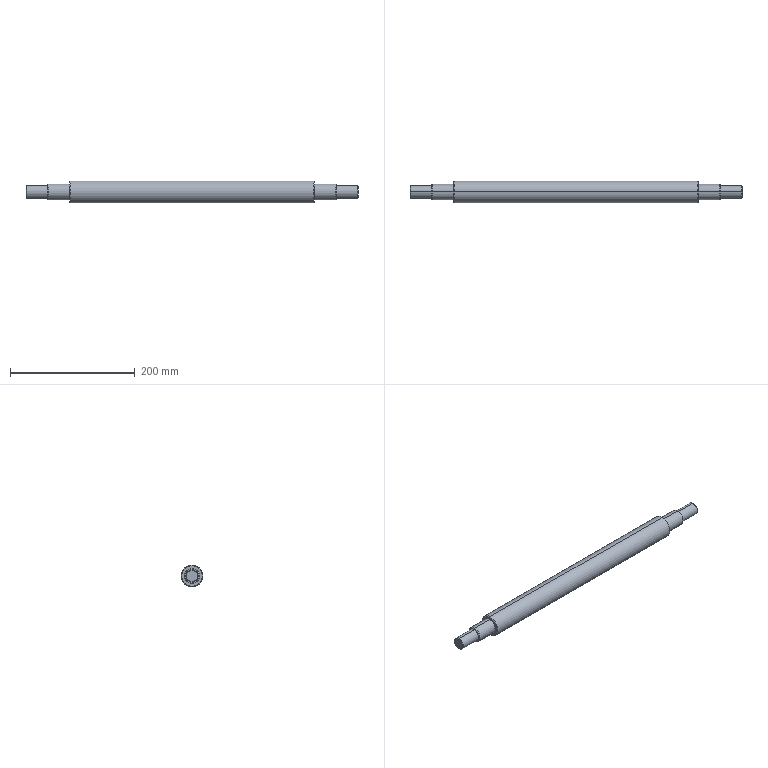Part | STEP file | Flat conveyor mechanism-CN2500x400-108-101 | 1 solid | 28 faces | box 532 x 35 x 35 mm | volume 433255 mm3 | cone 12 | cylinder 10 | plane 6 | commonest cylinder face diameters 20 x4 25 x4 35 x2
STEP:
#1=CARTESIAN_POINT('',(260.3,0.,-9.));
#2=VERTEX_POINT('',#1);
#3=CARTESIAN_POINT('',(260.3,0.,9.));
#4=VERTEX_POINT('',#3);
#5=CARTESIAN_POINT('',(260.3,0.,0.));
#6=DIRECTION('',(1.,0.,0.));
#7=DIRECTION('',(0.,0.,1.));
#8=AXIS2_PLACEMENT_3D('',#5,#6,#7);
#9=CIRCLE('',#8,9.);
#10=EDGE_CURVE('',#2,#4,#9,.T.);
#11=ORIENTED_EDGE('',*,*,#10,.F.);
#12=CARTESIAN_POINT('',(259.3,0.,-10.));
#13=VERTEX_POINT('',#12);
#14=CARTESIAN_POINT('',(259.3,0.,-10.));
#15=DIRECTION('',(-0.7071,0.,-0.7071));
#16=VECTOR('',#15,1000.);
#17=LINE('',#14,#16);
#18=EDGE_CURVE('',#2,#13,#17,.T.);
#19=ORIENTED_EDGE('',*,*,#18,.T.);
#20=CARTESIAN_POINT('',(259.3,0.,10.));
#21=VERTEX_POINT('',#20);
#22=CARTESIAN_POINT('',(259.3,0.,0.));
#23=DIRECTION('',(-1.,0.,0.));
#24=DIRECTION('',(0.,0.,1.));
#25=AXIS2_PLACEMENT_3D('',#22,#23,#24);
#26=CIRCLE('',#25,10.);
#27=EDGE_CURVE('',#21,#13,#26,.T.);
#28=ORIENTED_EDGE('',*,*,#27,.F.);
#29=CARTESIAN_POINT('',(259.3,0.,10.));
#30=DIRECTION('',(-0.7071,0.,0.7071));
#31=VECTOR('',#30,1000.);
#32=LINE('',#29,#31);
#33=EDGE_CURVE('',#4,#21,#32,.T.);
#34=ORIENTED_EDGE('',*,*,#33,.F.);
#35=EDGE_LOOP('',(#11,#19,#28,#34));
#36=FACE_OUTER_BOUND('',#35,.T.);
#37=CARTESIAN_POINT('',(259.3,0.,0.));
#38=DIRECTION('',(-1.,0.,0.));
#39=DIRECTION('',(0.,0.,1.));
#40=AXIS2_PLACEMENT_3D('',#37,#38,#39);
#41=CONICAL_SURFACE('',#40,10.,0.7854);
#42=ADVANCED_FACE('',(#36),#41,.T.);
#43=CARTESIAN_POINT('',(225.3,0.,-11.5));
#44=VERTEX_POINT('',#43);
#45=CARTESIAN_POINT('',(225.3,0.,11.5));
#46=VERTEX_POINT('',#45);
#47=CARTESIAN_POINT('',(225.3,0.,0.));
#48=DIRECTION('',(1.,0.,0.));
#49=DIRECTION('',(0.,0.,1.));
#50=AXIS2_PLACEMENT_3D('',#47,#48,#49);
#51=CIRCLE('',#50,11.5);
#52=EDGE_CURVE('',#44,#46,#51,.T.);
#53=ORIENTED_EDGE('',*,*,#52,.F.);
#54=CARTESIAN_POINT('',(224.3,0.,-12.5));
#55=VERTEX_POINT('',#54);
#56=CARTESIAN_POINT('',(224.3,0.,-12.5));
#57=DIRECTION('',(-0.7071,0.,-0.7071));
#58=VECTOR('',#57,1000.);
#59=LINE('',#56,#58);
#60=EDGE_CURVE('',#44,#55,#59,.T.);
#61=ORIENTED_EDGE('',*,*,#60,.T.);
#62=CARTESIAN_POINT('',(224.3,0.,12.5));
#63=VERTEX_POINT('',#62);
#64=CARTESIAN_POINT('',(224.3,0.,0.));
#65=DIRECTION('',(-1.,0.,0.));
#66=DIRECTION('',(0.,0.,1.));
#67=AXIS2_PLACEMENT_3D('',#64,#65,#66);
#68=CIRCLE('',#67,12.5);
#69=EDGE_CURVE('',#63,#55,#68,.T.);
#70=ORIENTED_EDGE('',*,*,#69,.F.);
#71=CARTESIAN_POINT('',(224.3,0.,12.5));
#72=DIRECTION('',(-0.7071,0.,0.7071));
#73=VECTOR('',#72,1000.);
#74=LINE('',#71,#73);
#75=EDGE_CURVE('',#46,#63,#74,.T.);
#76=ORIENTED_EDGE('',*,*,#75,.F.);
#77=EDGE_LOOP('',(#53,#61,#70,#76));
#78=FACE_OUTER_BOUND('',#77,.T.);
#79=CARTESIAN_POINT('',(224.3,0.,0.));
#80=DIRECTION('',(-1.,0.,0.));
#81=DIRECTION('',(0.,0.,1.));
#82=AXIS2_PLACEMENT_3D('',#79,#80,#81);
#83=CONICAL_SURFACE('',#82,12.5,0.7854);
#84=ADVANCED_FACE('',(#78),#83,.T.);
#85=CARTESIAN_POINT('',(190.3,0.,-16.5));
#86=VERTEX_POINT('',#85);
#87=CARTESIAN_POINT('',(190.3,0.,16.5));
#88=VERTEX_POINT('',#87);
#89=CARTESIAN_POINT('',(190.3,0.,0.));
#90=DIRECTION('',(1.,0.,0.));
#91=DIRECTION('',(0.,0.,1.));
#92=AXIS2_PLACEMENT_3D('',#89,#90,#91);
#93=CIRCLE('',#92,16.5);
#94=EDGE_CURVE('',#86,#88,#93,.T.);
#95=ORIENTED_EDGE('',*,*,#94,.F.);
#96=CARTESIAN_POINT('',(189.3,0.,-17.5));
#97=VERTEX_POINT('',#96);
#98=CARTESIAN_POINT('',(189.3,0.,-17.5));
#99=DIRECTION('',(-0.7071,0.,-0.7071));
#100=VECTOR('',#99,1000.);
#101=LINE('',#98,#100);
#102=EDGE_CURVE('',#86,#97,#101,.T.);
#103=ORIENTED_EDGE('',*,*,#102,.T.);
#104=CARTESIAN_POINT('',(189.3,0.,17.5));
#105=VERTEX_POINT('',#104);
#106=CARTESIAN_POINT('',(189.3,0.,0.));
#107=DIRECTION('',(-1.,0.,0.));
#108=DIRECTION('',(0.,0.,1.));
#109=AXIS2_PLACEMENT_3D('',#106,#107,#108);
#110=CIRCLE('',#109,17.5);
#111=EDGE_CURVE('',#105,#97,#110,.T.);
#112=ORIENTED_EDGE('',*,*,#111,.F.);
#113=CARTESIAN_POINT('',(189.3,0.,17.5));
#114=DIRECTION('',(-0.7071,0.,0.7071));
#115=VECTOR('',#114,1000.);
#116=LINE('',#113,#115);
#117=EDGE_CURVE('',#88,#105,#116,.T.);
#118=ORIENTED_EDGE('',*,*,#117,.F.);
#119=EDGE_LOOP('',(#95,#103,#112,#118));
#120=FACE_OUTER_BOUND('',#119,.T.);
#121=CARTESIAN_POINT('',(189.3,0.,0.));
#122=DIRECTION('',(-1.,0.,0.));
#123=DIRECTION('',(0.,0.,1.));
#124=AXIS2_PLACEMENT_3D('',#121,#122,#123);
#125=CONICAL_SURFACE('',#124,17.5,0.7854);
#126=ADVANCED_FACE('',(#120),#125,.T.);
#127=CARTESIAN_POINT('',(-201.7,0.,16.5));
#128=VERTEX_POINT('',#127);
#129=CARTESIAN_POINT('',(-201.7,0.,-16.5));
#130=VERTEX_POINT('',#129);
#131=CARTESIAN_POINT('',(-201.7,0.,0.));
#132=DIRECTION('',(-1.,0.,0.));
#133=DIRECTION('',(0.,0.,-1.));
#134=AXIS2_PLACEMENT_3D('',#131,#132,#133);
#135=CIRCLE('',#134,16.5);
#136=EDGE_CURVE('',#128,#130,#135,.T.);
#137=ORIENTED_EDGE('',*,*,#136,.F.);
#138=CARTESIAN_POINT('',(-200.7,0.,17.5));
#139=VERTEX_POINT('',#138);
#140=CARTESIAN_POINT('',(-201.7,0.,16.5));
#141=DIRECTION('',(0.7071,0.,0.7071));
#142=VECTOR('',#141,1000.);
#143=LINE('',#140,#142);
#144=EDGE_CURVE('',#128,#139,#143,.T.);
#145=ORIENTED_EDGE('',*,*,#144,.T.);
#146=CARTESIAN_POINT('',(-200.7,0.,-17.5));
#147=VERTEX_POINT('',#146);
#148=CARTESIAN_POINT('',(-200.7,0.,0.));
#149=DIRECTION('',(1.,0.,0.));
#150=DIRECTION('',(0.,0.,-1.));
#151=AXIS2_PLACEMENT_3D('',#148,#149,#150);
#152=CIRCLE('',#151,17.5);
#153=EDGE_CURVE('',#147,#139,#152,.T.);
#154=ORIENTED_EDGE('',*,*,#153,.F.);
#155=CARTESIAN_POINT('',(-201.7,0.,-16.5));
#156=DIRECTION('',(0.7071,0.,-0.7071));
#157=VECTOR('',#156,1000.);
#158=LINE('',#155,#157);
#159=EDGE_CURVE('',#130,#147,#158,.T.);
#160=ORIENTED_EDGE('',*,*,#159,.F.);
#161=EDGE_LOOP('',(#137,#145,#154,#160));
#162=FACE_OUTER_BOUND('',#161,.T.);
#163=CARTESIAN_POINT('',(-201.7,0.,0.));
#164=DIRECTION('',(1.,0.,0.));
#165=DIRECTION('',(0.,0.,-1.));
#166=AXIS2_PLACEMENT_3D('',#163,#164,#165);
#167=CONICAL_SURFACE('',#166,16.5,0.7854);
#168=ADVANCED_FACE('',(#162),#167,.T.);
#169=CARTESIAN_POINT('',(-236.7,0.,11.5));
#170=VERTEX_POINT('',#169);
#171=CARTESIAN_POINT('',(-236.7,0.,-11.5));
#172=VERTEX_POINT('',#171);
#173=CARTESIAN_POINT('',(-236.7,0.,0.));
#174=DIRECTION('',(-1.,0.,0.));
#175=DIRECTION('',(0.,0.,-1.));
#176=AXIS2_PLACEMENT_3D('',#173,#174,#175);
#177=CIRCLE('',#176,11.5);
#178=EDGE_CURVE('',#170,#172,#177,.T.);
#179=ORIENTED_EDGE('',*,*,#178,.F.);
#180=CARTESIAN_POINT('',(-235.7,0.,12.5));
#181=VERTEX_POINT('',#180);
#182=CARTESIAN_POINT('',(-236.7,0.,11.5));
#183=DIRECTION('',(0.7071,0.,0.7071));
#184=VECTOR('',#183,1000.);
#185=LINE('',#182,#184);
#186=EDGE_CURVE('',#170,#181,#185,.T.);
#187=ORIENTED_EDGE('',*,*,#186,.T.);
#188=CARTESIAN_POINT('',(-235.7,0.,-12.5));
#189=VERTEX_POINT('',#188);
#190=CARTESIAN_POINT('',(-235.7,0.,0.));
#191=DIRECTION('',(1.,0.,0.));
#192=DIRECTION('',(0.,0.,-1.));
#193=AXIS2_PLACEMENT_3D('',#190,#191,#192);
#194=CIRCLE('',#193,12.5);
#195=EDGE_CURVE('',#189,#181,#194,.T.);
#196=ORIENTED_EDGE('',*,*,#195,.F.);
#197=CARTESIAN_POINT('',(-236.7,0.,-11.5));
#198=DIRECTION('',(0.7071,0.,-0.7071));
#199=VECTOR('',#198,1000.);
#200=LINE('',#197,#199);
#201=EDGE_CURVE('',#172,#189,#200,.T.);
#202=ORIENTED_EDGE('',*,*,#201,.F.);
#203=EDGE_LOOP('',(#179,#187,#196,#202));
#204=FACE_OUTER_BOUND('',#203,.T.);
#205=CARTESIAN_POINT('',(-236.7,0.,0.));
#206=DIRECTION('',(1.,0.,0.));
#207=DIRECTION('',(0.,0.,-1.));
#208=AXIS2_PLACEMENT_3D('',#205,#206,#207);
#209=CONICAL_SURFACE('',#208,11.5,0.7854);
#210=ADVANCED_FACE('',(#204),#209,.T.);
#211=CARTESIAN_POINT('',(-271.7,0.,9.));
#212=VERTEX_POINT('',#211);
#213=CARTESIAN_POINT('',(-271.7,0.,-9.));
#214=VERTEX_POINT('',#213);
#215=CARTESIAN_POINT('',(-271.7,0.,0.));
#216=DIRECTION('',(-1.,0.,0.));
#217=DIRECTION('',(0.,0.,-1.));
#218=AXIS2_PLACEMENT_3D('',#215,#216,#217);
#219=CIRCLE('',#218,9.);
#220=EDGE_CURVE('',#212,#214,#219,.T.);
#221=ORIENTED_EDGE('',*,*,#220,.F.);
#222=CARTESIAN_POINT('',(-270.7,0.,10.));
#223=VERTEX_POINT('',#222);
#224=CARTESIAN_POINT('',(-271.7,0.,9.));
#225=DIRECTION('',(0.7071,0.,0.7071));
#226=VECTOR('',#225,1000.);
#227=LINE('',#224,#226);
#228=EDGE_CURVE('',#212,#223,#227,.T.);
#229=ORIENTED_EDGE('',*,*,#228,.T.);
#230=CARTESIAN_POINT('',(-270.7,0.,-10.));
#231=VERTEX_POINT('',#230);
#232=CARTESIAN_POINT('',(-270.7,0.,0.));
#233=DIRECTION('',(1.,0.,0.));
#234=DIRECTION('',(0.,0.,-1.));
#235=AXIS2_PLACEMENT_3D('',#232,#233,#234);
#236=CIRCLE('',#235,10.);
#237=EDGE_CURVE('',#231,#223,#236,.T.);
#238=ORIENTED_EDGE('',*,*,#237,.F.);
#239=CARTESIAN_POINT('',(-271.7,0.,-9.));
#240=DIRECTION('',(0.7071,0.,-0.7071));
#241=VECTOR('',#240,1000.);
#242=LINE('',#239,#241);
#243=EDGE_CURVE('',#214,#231,#242,.T.);
#244=ORIENTED_EDGE('',*,*,#243,.F.);
#245=EDGE_LOOP('',(#221,#229,#238,#244));
#246=FACE_OUTER_BOUND('',#245,.T.);
#247=CARTESIAN_POINT('',(-271.7,0.,0.));
#248=DIRECTION('',(1.,0.,0.));
#249=DIRECTION('',(0.,0.,-1.));
#250=AXIS2_PLACEMENT_3D('',#247,#248,#249);
#251=CONICAL_SURFACE('',#250,9.,0.7854);
#252=ADVANCED_FACE('',(#246),#251,.T.);
#253=ORIENTED_EDGE('',*,*,#27,.T.);
#254=CARTESIAN_POINT('',(225.3,0.,-10.));
#255=VERTEX_POINT('',#254);
#256=CARTESIAN_POINT('',(-209.5,0.,-10.));
#257=DIRECTION('',(-1.,0.,0.));
#258=VECTOR('',#257,1000.);
#259=LINE('',#256,#258);
#260=EDGE_CURVE('',#13,#255,#259,.T.);
#261=ORIENTED_EDGE('',*,*,#260,.T.);
#262=CARTESIAN_POINT('',(225.3,0.,10.));
#263=VERTEX_POINT('',#262);
#264=CARTESIAN_POINT('',(225.3,0.,0.));
#265=DIRECTION('',(-1.,0.,0.));
#266=DIRECTION('',(0.,0.,1.));
#267=AXIS2_PLACEMENT_3D('',#264,#265,#266);
#268=CIRCLE('',#267,10.);
#269=EDGE_CURVE('',#263,#255,#268,.T.);
#270=ORIENTED_EDGE('',*,*,#269,.F.);
#271=CARTESIAN_POINT('',(-209.5,0.,10.));
#272=DIRECTION('',(-1.,0.,0.));
#273=VECTOR('',#272,1000.);
#274=LINE('',#271,#273);
#275=EDGE_CURVE('',#21,#263,#274,.T.);
#276=ORIENTED_EDGE('',*,*,#275,.F.);
#277=EDGE_LOOP('',(#253,#261,#270,#276));
#278=FACE_OUTER_BOUND('',#277,.T.);
#279=CARTESIAN_POINT('',(-209.5,0.,0.));
#280=DIRECTION('',(-1.,0.,0.));
#281=DIRECTION('',(0.,0.,1.));
#282=AXIS2_PLACEMENT_3D('',#279,#280,#281);
#283=CYLINDRICAL_SURFACE('',#282,10.);
#284=ADVANCED_FACE('',(#278),#283,.T.);
#285=ORIENTED_EDGE('',*,*,#69,.T.);
#286=CARTESIAN_POINT('',(190.3,0.,-12.5));
#287=VERTEX_POINT('',#286);
#288=CARTESIAN_POINT('',(-209.5,0.,-12.5));
#289=DIRECTION('',(-1.,0.,0.));
#290=VECTOR('',#289,1000.);
#291=LINE('',#288,#290);
#292=EDGE_CURVE('',#55,#287,#291,.T.);
#293=ORIENTED_EDGE('',*,*,#292,.T.);
#294=CARTESIAN_POINT('',(190.3,0.,12.5));
#295=VERTEX_POINT('',#294);
#296=CARTESIAN_POINT('',(190.3,0.,0.));
#297=DIRECTION('',(-1.,0.,0.));
#298=DIRECTION('',(0.,0.,1.));
#299=AXIS2_PLACEMENT_3D('',#296,#297,#298);
#300=CIRCLE('',#299,12.5);
#301=EDGE_CURVE('',#295,#287,#300,.T.);
#302=ORIENTED_EDGE('',*,*,#301,.F.);
#303=CARTESIAN_POINT('',(-209.5,0.,12.5));
#304=DIRECTION('',(-1.,0.,0.));
#305=VECTOR('',#304,1000.);
#306=LINE('',#303,#305);
#307=EDGE_CURVE('',#63,#295,#306,.T.);
#308=ORIENTED_EDGE('',*,*,#307,.F.);
#309=EDGE_LOOP('',(#285,#293,#302,#308));
#310=FACE_OUTER_BOUND('',#309,.T.);
#311=CARTESIAN_POINT('',(-209.5,0.,0.));
#312=DIRECTION('',(-1.,0.,0.));
#313=DIRECTION('',(0.,0.,1.));
#314=AXIS2_PLACEMENT_3D('',#311,#312,#313);
#315=CYLINDRICAL_SURFACE('',#314,12.5);
#316=ADVANCED_FACE('',(#310),#315,.T.);
#317=ORIENTED_EDGE('',*,*,#111,.T.);
#318=CARTESIAN_POINT('',(-209.5,0.,-17.5));
#319=DIRECTION('',(-1.,0.,0.));
#320=VECTOR('',#319,1000.);
#321=LINE('',#318,#320);
#322=EDGE_CURVE('',#97,#147,#321,.T.);
#323=ORIENTED_EDGE('',*,*,#322,.T.);
#324=ORIENTED_EDGE('',*,*,#153,.T.);
#325=CARTESIAN_POINT('',(-209.5,0.,17.5));
#326=DIRECTION('',(-1.,0.,0.));
#327=VECTOR('',#326,1000.);
#328=LINE('',#325,#327);
#329=EDGE_CURVE('',#105,#139,#328,.T.);
#330=ORIENTED_EDGE('',*,*,#329,.F.);
#331=EDGE_LOOP('',(#317,#323,#324,#330));
#332=FACE_OUTER_BOUND('',#331,.T.);
#333=CARTESIAN_POINT('',(-209.5,0.,0.));
#334=DIRECTION('',(-1.,0.,0.));
#335=DIRECTION('',(0.,0.,1.));
#336=AXIS2_PLACEMENT_3D('',#333,#334,#335);
#337=CYLINDRICAL_SURFACE('',#336,17.5);
#338=ADVANCED_FACE('',(#332),#337,.T.);
#339=CARTESIAN_POINT('',(-201.7,0.,12.5));
#340=VERTEX_POINT('',#339);
#341=CARTESIAN_POINT('',(-201.7,0.,-12.5));
#342=VERTEX_POINT('',#341);
#343=CARTESIAN_POINT('',(-201.7,0.,0.));
#344=DIRECTION('',(-1.,0.,0.));
#345=DIRECTION('',(0.,0.,1.));
#346=AXIS2_PLACEMENT_3D('',#343,#344,#345);
#347=CIRCLE('',#346,12.5);
#348=EDGE_CURVE('',#340,#342,#347,.T.);
#349=ORIENTED_EDGE('',*,*,#348,.T.);
#350=CARTESIAN_POINT('',(-209.5,0.,-12.5));
#351=DIRECTION('',(-1.,0.,0.));
#352=VECTOR('',#351,1000.);
#353=LINE('',#350,#352);
#354=EDGE_CURVE('',#342,#189,#353,.T.);
#355=ORIENTED_EDGE('',*,*,#354,.T.);
#356=ORIENTED_EDGE('',*,*,#195,.T.);
#357=CARTESIAN_POINT('',(-209.5,0.,12.5));
#358=DIRECTION('',(-1.,0.,0.));
#359=VECTOR('',#358,1000.);
#360=LINE('',#357,#359);
#361=EDGE_CURVE('',#340,#181,#360,.T.);
#362=ORIENTED_EDGE('',*,*,#361,.F.);
#363=EDGE_LOOP('',(#349,#355,#356,#362));
#364=FACE_OUTER_BOUND('',#363,.T.);
#365=CARTESIAN_POINT('',(-209.5,0.,0.));
#366=DIRECTION('',(-1.,0.,0.));
#367=DIRECTION('',(0.,0.,1.));
#368=AXIS2_PLACEMENT_3D('',#365,#366,#367);
#369=CYLINDRICAL_SURFACE('',#368,12.5);
#370=ADVANCED_FACE('',(#364),#369,.T.);
#371=CARTESIAN_POINT('',(-236.7,0.,10.));
#372=VERTEX_POINT('',#371);
#373=CARTESIAN_POINT('',(-236.7,0.,-10.));
#374=VERTEX_POINT('',#373);
#375=CARTESIAN_POINT('',(-236.7,0.,0.));
#376=DIRECTION('',(-1.,0.,0.));
#377=DIRECTION('',(0.,0.,1.));
#378=AXIS2_PLACEMENT_3D('',#375,#376,#377);
#379=CIRCLE('',#378,10.);
#380=EDGE_CURVE('',#372,#374,#379,.T.);
#381=ORIENTED_EDGE('',*,*,#380,.T.);
#382=CARTESIAN_POINT('',(-209.5,0.,-10.));
#383=DIRECTION('',(-1.,0.,0.));
#384=VECTOR('',#383,1000.);
#385=LINE('',#382,#384);
#386=EDGE_CURVE('',#374,#231,#385,.T.);
#387=ORIENTED_EDGE('',*,*,#386,.T.);
#388=ORIENTED_EDGE('',*,*,#237,.T.);
#389=CARTESIAN_POINT('',(-209.5,0.,10.));
#390=DIRECTION('',(-1.,0.,0.));
#391=VECTOR('',#390,1000.);
#392=LINE('',#389,#391);
#393=EDGE_CURVE('',#372,#223,#392,.T.);
#394=ORIENTED_EDGE('',*,*,#393,.F.);
#395=EDGE_LOOP('',(#381,#387,#388,#394));
#396=FACE_OUTER_BOUND('',#395,.T.);
#397=CARTESIAN_POINT('',(-209.5,0.,0.));
#398=DIRECTION('',(-1.,0.,0.));
#399=DIRECTION('',(0.,0.,1.));
#400=AXIS2_PLACEMENT_3D('',#397,#398,#399);
#401=CYLINDRICAL_SURFACE('',#400,10.);
#402=ADVANCED_FACE('',(#396),#401,.T.);
#403=CARTESIAN_POINT('',(-271.7,0.,0.));
#404=DIRECTION('',(-1.,0.,0.));
#405=DIRECTION('',(0.,0.,-1.));
#406=AXIS2_PLACEMENT_3D('',#403,#404,#405);
#407=CIRCLE('',#406,9.);
#408=EDGE_CURVE('',#214,#212,#407,.T.);
#409=ORIENTED_EDGE('',*,*,#408,.T.);
#410=ORIENTED_EDGE('',*,*,#220,.T.);
#411=EDGE_LOOP('',(#409,#410));
#412=FACE_OUTER_BOUND('',#411,.T.);
#413=CARTESIAN_POINT('',(-271.7,10.,0.));
#414=DIRECTION('',(1.,0.,0.));
#415=DIRECTION('',(0.,0.,-1.));
#416=AXIS2_PLACEMENT_3D('',#413,#414,#415);
#417=PLANE('',#416);
#418=ADVANCED_FACE('',(#412),#417,.F.);
#419=ORIENTED_EDGE('',*,*,#386,.F.);
#420=CARTESIAN_POINT('',(-236.7,0.,0.));
#421=DIRECTION('',(-1.,0.,0.));
#422=DIRECTION('',(0.,0.,1.));
#423=AXIS2_PLACEMENT_3D('',#420,#421,#422);
#424=CIRCLE('',#423,10.);
#425=EDGE_CURVE('',#374,#372,#424,.T.);
#426=ORIENTED_EDGE('',*,*,#425,.T.);
#427=ORIENTED_EDGE('',*,*,#393,.T.);
#428=CARTESIAN_POINT('',(-270.7,0.,0.));
#429=DIRECTION('',(1.,0.,0.));
#430=DIRECTION('',(0.,0.,-1.));
#431=AXIS2_PLACEMENT_3D('',#428,#429,#430);
#432=CIRCLE('',#431,10.);
#433=EDGE_CURVE('',#223,#231,#432,.T.);
#434=ORIENTED_EDGE('',*,*,#433,.T.);
#435=EDGE_LOOP('',(#419,#426,#427,#434));
#436=FACE_OUTER_BOUND('',#435,.T.);
#437=CARTESIAN_POINT('',(-209.5,0.,0.));
#438=DIRECTION('',(-1.,0.,0.));
#439=DIRECTION('',(0.,0.,1.));
#440=AXIS2_PLACEMENT_3D('',#437,#438,#439);
#441=CYLINDRICAL_SURFACE('',#440,10.);
#442=ADVANCED_FACE('',(#436),#441,.T.);
#443=CARTESIAN_POINT('',(-236.7,0.,0.));
#444=DIRECTION('',(-1.,0.,0.));
#445=DIRECTION('',(0.,0.,-1.));
#446=AXIS2_PLACEMENT_3D('',#443,#444,#445);
#447=CIRCLE('',#446,11.5);
#448=EDGE_CURVE('',#172,#170,#447,.T.);
#449=ORIENTED_EDGE('',*,*,#448,.T.);
#450=ORIENTED_EDGE('',*,*,#178,.T.);
#451=EDGE_LOOP('',(#449,#450));
#452=FACE_OUTER_BOUND('',#451,.T.);
#453=ORIENTED_EDGE('',*,*,#380,.F.);
#454=ORIENTED_EDGE('',*,*,#425,.F.);
#455=EDGE_LOOP('',(#453,#454));
#456=FACE_BOUND('',#455,.T.);
#457=CARTESIAN_POINT('',(-236.7,12.5,0.));
#458=DIRECTION('',(1.,0.,0.));
#459=DIRECTION('',(0.,0.,-1.));
#460=AXIS2_PLACEMENT_3D('',#457,#458,#459);
#461=PLANE('',#460);
#462=ADVANCED_FACE('',(#452,#456),#461,.F.);
#463=ORIENTED_EDGE('',*,*,#354,.F.);
#464=CARTESIAN_POINT('',(-201.7,0.,0.));
#465=DIRECTION('',(-1.,0.,0.));
#466=DIRECTION('',(0.,0.,1.));
#467=AXIS2_PLACEMENT_3D('',#464,#465,#466);
#468=CIRCLE('',#467,12.5);
#469=EDGE_CURVE('',#342,#340,#468,.T.);
#470=ORIENTED_EDGE('',*,*,#469,.T.);
#471=ORIENTED_EDGE('',*,*,#361,.T.);
#472=CARTESIAN_POINT('',(-235.7,0.,0.));
#473=DIRECTION('',(1.,0.,0.));
#474=DIRECTION('',(0.,0.,-1.));
#475=AXIS2_PLACEMENT_3D('',#472,#473,#474);
#476=CIRCLE('',#475,12.5);
#477=EDGE_CURVE('',#181,#189,#476,.T.);
#478=ORIENTED_EDGE('',*,*,#477,.T.);
#479=EDGE_LOOP('',(#463,#470,#471,#478));
#480=FACE_OUTER_BOUND('',#479,.T.);
#481=CARTESIAN_POINT('',(-209.5,0.,0.));
#482=DIRECTION('',(-1.,0.,0.));
#483=DIRECTION('',(0.,0.,1.));
#484=AXIS2_PLACEMENT_3D('',#481,#482,#483);
#485=CYLINDRICAL_SURFACE('',#484,12.5);
#486=ADVANCED_FACE('',(#480),#485,.T.);
#487=CARTESIAN_POINT('',(-201.7,0.,0.));
#488=DIRECTION('',(-1.,0.,0.));
#489=DIRECTION('',(0.,0.,-1.));
#490=AXIS2_PLACEMENT_3D('',#487,#488,#489);
#491=CIRCLE('',#490,16.5);
#492=EDGE_CURVE('',#130,#128,#491,.T.);
#493=ORIENTED_EDGE('',*,*,#492,.T.);
#494=ORIENTED_EDGE('',*,*,#136,.T.);
#495=EDGE_LOOP('',(#493,#494));
#496=FACE_OUTER_BOUND('',#495,.T.);
#497=ORIENTED_EDGE('',*,*,#348,.F.);
#498=ORIENTED_EDGE('',*,*,#469,.F.);
#499=EDGE_LOOP('',(#497,#498));
#500=FACE_BOUND('',#499,.T.);
#501=CARTESIAN_POINT('',(-201.7,17.5,0.));
#502=DIRECTION('',(1.,0.,0.));
#503=DIRECTION('',(0.,0.,-1.));
#504=AXIS2_PLACEMENT_3D('',#501,#502,#503);
#505=PLANE('',#504);
#506=ADVANCED_FACE('',(#496,#500),#505,.F.);
#507=ORIENTED_EDGE('',*,*,#322,.F.);
#508=CARTESIAN_POINT('',(189.3,0.,0.));
#509=DIRECTION('',(-1.,0.,0.));
#510=DIRECTION('',(0.,0.,1.));
#511=AXIS2_PLACEMENT_3D('',#508,#509,#510);
#512=CIRCLE('',#511,17.5);
#513=EDGE_CURVE('',#97,#105,#512,.T.);
#514=ORIENTED_EDGE('',*,*,#513,.T.);
#515=ORIENTED_EDGE('',*,*,#329,.T.);
#516=CARTESIAN_POINT('',(-200.7,0.,0.));
#517=DIRECTION('',(1.,0.,0.));
#518=DIRECTION('',(0.,0.,-1.));
#519=AXIS2_PLACEMENT_3D('',#516,#517,#518);
#520=CIRCLE('',#519,17.5);
#521=EDGE_CURVE('',#139,#147,#520,.T.);
#522=ORIENTED_EDGE('',*,*,#521,.T.);
#523=EDGE_LOOP('',(#507,#514,#515,#522));
#524=FACE_OUTER_BOUND('',#523,.T.);
#525=CARTESIAN_POINT('',(-209.5,0.,0.));
#526=DIRECTION('',(-1.,0.,0.));
#527=DIRECTION('',(0.,0.,1.));
#528=AXIS2_PLACEMENT_3D('',#525,#526,#527);
#529=CYLINDRICAL_SURFACE('',#528,17.5);
#530=ADVANCED_FACE('',(#524),#529,.T.);
#531=CARTESIAN_POINT('',(190.3,0.,0.));
#532=DIRECTION('',(1.,0.,0.));
#533=DIRECTION('',(0.,0.,1.));
#534=AXIS2_PLACEMENT_3D('',#531,#532,#533);
#535=CIRCLE('',#534,16.5);
#536=EDGE_CURVE('',#88,#86,#535,.T.);
#537=ORIENTED_EDGE('',*,*,#536,.T.);
#538=ORIENTED_EDGE('',*,*,#94,.T.);
#539=EDGE_LOOP('',(#537,#538));
#540=FACE_OUTER_BOUND('',#539,.T.);
#541=ORIENTED_EDGE('',*,*,#301,.T.);
#542=CARTESIAN_POINT('',(190.3,0.,0.));
#543=DIRECTION('',(-1.,0.,0.));
#544=DIRECTION('',(0.,0.,1.));
#545=AXIS2_PLACEMENT_3D('',#542,#543,#544);
#546=CIRCLE('',#545,12.5);
#547=EDGE_CURVE('',#287,#295,#546,.T.);
#548=ORIENTED_EDGE('',*,*,#547,.T.);
#549=EDGE_LOOP('',(#541,#548));
#550=FACE_BOUND('',#549,.T.);
#551=CARTESIAN_POINT('',(190.3,12.5,0.));
#552=DIRECTION('',(-1.,0.,0.));
#553=DIRECTION('',(0.,0.,1.));
#554=AXIS2_PLACEMENT_3D('',#551,#552,#553);
#555=PLANE('',#554);
#556=ADVANCED_FACE('',(#540,#550),#555,.F.);
#557=ORIENTED_EDGE('',*,*,#292,.F.);
#558=CARTESIAN_POINT('',(224.3,0.,0.));
#559=DIRECTION('',(-1.,0.,0.));
#560=DIRECTION('',(0.,0.,1.));
#561=AXIS2_PLACEMENT_3D('',#558,#559,#560);
#562=CIRCLE('',#561,12.5);
#563=EDGE_CURVE('',#55,#63,#562,.T.);
#564=ORIENTED_EDGE('',*,*,#563,.T.);
#565=ORIENTED_EDGE('',*,*,#307,.T.);
#566=ORIENTED_EDGE('',*,*,#547,.F.);
#567=EDGE_LOOP('',(#557,#564,#565,#566));
#568=FACE_OUTER_BOUND('',#567,.T.);
#569=CARTESIAN_POINT('',(-209.5,0.,0.));
#570=DIRECTION('',(-1.,0.,0.));
#571=DIRECTION('',(0.,0.,1.));
#572=AXIS2_PLACEMENT_3D('',#569,#570,#571);
#573=CYLINDRICAL_SURFACE('',#572,12.5);
#574=ADVANCED_FACE('',(#568),#573,.T.);
#575=CARTESIAN_POINT('',(225.3,0.,0.));
#576=DIRECTION('',(1.,0.,0.));
#577=DIRECTION('',(0.,0.,1.));
#578=AXIS2_PLACEMENT_3D('',#575,#576,#577);
#579=CIRCLE('',#578,11.5);
#580=EDGE_CURVE('',#46,#44,#579,.T.);
#581=ORIENTED_EDGE('',*,*,#580,.T.);
#582=ORIENTED_EDGE('',*,*,#52,.T.);
#583=EDGE_LOOP('',(#581,#582));
#584=FACE_OUTER_BOUND('',#583,.T.);
#585=ORIENTED_EDGE('',*,*,#269,.T.);
#586=CARTESIAN_POINT('',(225.3,0.,0.));
#587=DIRECTION('',(-1.,0.,0.));
#588=DIRECTION('',(0.,0.,1.));
#589=AXIS2_PLACEMENT_3D('',#586,#587,#588);
#590=CIRCLE('',#589,10.);
#591=EDGE_CURVE('',#255,#263,#590,.T.);
#592=ORIENTED_EDGE('',*,*,#591,.T.);
#593=EDGE_LOOP('',(#585,#592));
#594=FACE_BOUND('',#593,.T.);
#595=CARTESIAN_POINT('',(225.3,12.5,0.));
#596=DIRECTION('',(-1.,0.,0.));
#597=DIRECTION('',(0.,0.,1.));
#598=AXIS2_PLACEMENT_3D('',#595,#596,#597);
#599=PLANE('',#598);
#600=ADVANCED_FACE('',(#584,#594),#599,.F.);
#601=ORIENTED_EDGE('',*,*,#260,.F.);
#602=CARTESIAN_POINT('',(259.3,0.,0.));
#603=DIRECTION('',(-1.,0.,0.));
#604=DIRECTION('',(0.,0.,1.));
#605=AXIS2_PLACEMENT_3D('',#602,#603,#604);
#606=CIRCLE('',#605,10.);
#607=EDGE_CURVE('',#13,#21,#606,.T.);
#608=ORIENTED_EDGE('',*,*,#607,.T.);
#609=ORIENTED_EDGE('',*,*,#275,.T.);
#610=ORIENTED_EDGE('',*,*,#591,.F.);
#611=EDGE_LOOP('',(#601,#608,#609,#610));
#612=FACE_OUTER_BOUND('',#611,.T.);
#613=CARTESIAN_POINT('',(-209.5,0.,0.));
#614=DIRECTION('',(-1.,0.,0.));
#615=DIRECTION('',(0.,0.,1.));
#616=AXIS2_PLACEMENT_3D('',#613,#614,#615);
#617=CYLINDRICAL_SURFACE('',#616,10.);
#618=ADVANCED_FACE('',(#612),#617,.T.);
#619=CARTESIAN_POINT('',(260.3,0.,0.));
#620=DIRECTION('',(1.,0.,0.));
#621=DIRECTION('',(0.,0.,1.));
#622=AXIS2_PLACEMENT_3D('',#619,#620,#621);
#623=CIRCLE('',#622,9.);
#624=EDGE_CURVE('',#4,#2,#623,.T.);
#625=ORIENTED_EDGE('',*,*,#624,.T.);
#626=ORIENTED_EDGE('',*,*,#10,.T.);
#627=EDGE_LOOP('',(#625,#626));
#628=FACE_OUTER_BOUND('',#627,.T.);
#629=CARTESIAN_POINT('',(260.3,10.,0.));
#630=DIRECTION('',(-1.,0.,0.));
#631=DIRECTION('',(0.,0.,1.));
#632=AXIS2_PLACEMENT_3D('',#629,#630,#631);
#633=PLANE('',#632);
#634=ADVANCED_FACE('',(#628),#633,.F.);
#635=ORIENTED_EDGE('',*,*,#228,.F.);
#636=ORIENTED_EDGE('',*,*,#408,.F.);
#637=ORIENTED_EDGE('',*,*,#243,.T.);
#638=ORIENTED_EDGE('',*,*,#433,.F.);
#639=EDGE_LOOP('',(#635,#636,#637,#638));
#640=FACE_OUTER_BOUND('',#639,.T.);
#641=CARTESIAN_POINT('',(-271.7,0.,0.));
#642=DIRECTION('',(1.,0.,0.));
#643=DIRECTION('',(0.,0.,-1.));
#644=AXIS2_PLACEMENT_3D('',#641,#642,#643);
#645=CONICAL_SURFACE('',#644,9.,0.7854);
#646=ADVANCED_FACE('',(#640),#645,.T.);
#647=ORIENTED_EDGE('',*,*,#186,.F.);
#648=ORIENTED_EDGE('',*,*,#448,.F.);
#649=ORIENTED_EDGE('',*,*,#201,.T.);
#650=ORIENTED_EDGE('',*,*,#477,.F.);
#651=EDGE_LOOP('',(#647,#648,#649,#650));
#652=FACE_OUTER_BOUND('',#651,.T.);
#653=CARTESIAN_POINT('',(-236.7,0.,0.));
#654=DIRECTION('',(1.,0.,0.));
#655=DIRECTION('',(0.,0.,-1.));
#656=AXIS2_PLACEMENT_3D('',#653,#654,#655);
#657=CONICAL_SURFACE('',#656,11.5,0.7854);
#658=ADVANCED_FACE('',(#652),#657,.T.);
#659=ORIENTED_EDGE('',*,*,#144,.F.);
#660=ORIENTED_EDGE('',*,*,#492,.F.);
#661=ORIENTED_EDGE('',*,*,#159,.T.);
#662=ORIENTED_EDGE('',*,*,#521,.F.);
#663=EDGE_LOOP('',(#659,#660,#661,#662));
#664=FACE_OUTER_BOUND('',#663,.T.);
#665=CARTESIAN_POINT('',(-201.7,0.,0.));
#666=DIRECTION('',(1.,0.,0.));
#667=DIRECTION('',(0.,0.,-1.));
#668=AXIS2_PLACEMENT_3D('',#665,#666,#667);
#669=CONICAL_SURFACE('',#668,16.5,0.7854);
#670=ADVANCED_FACE('',(#664),#669,.T.);
#671=ORIENTED_EDGE('',*,*,#102,.F.);
#672=ORIENTED_EDGE('',*,*,#536,.F.);
#673=ORIENTED_EDGE('',*,*,#117,.T.);
#674=ORIENTED_EDGE('',*,*,#513,.F.);
#675=EDGE_LOOP('',(#671,#672,#673,#674));
#676=FACE_OUTER_BOUND('',#675,.T.);
#677=CARTESIAN_POINT('',(189.3,0.,0.));
#678=DIRECTION('',(-1.,0.,0.));
#679=DIRECTION('',(0.,0.,1.));
#680=AXIS2_PLACEMENT_3D('',#677,#678,#679);
#681=CONICAL_SURFACE('',#680,17.5,0.7854);
#682=ADVANCED_FACE('',(#676),#681,.T.);
#683=ORIENTED_EDGE('',*,*,#60,.F.);
#684=ORIENTED_EDGE('',*,*,#580,.F.);
#685=ORIENTED_EDGE('',*,*,#75,.T.);
#686=ORIENTED_EDGE('',*,*,#563,.F.);
#687=EDGE_LOOP('',(#683,#684,#685,#686));
#688=FACE_OUTER_BOUND('',#687,.T.);
#689=CARTESIAN_POINT('',(224.3,0.,0.));
#690=DIRECTION('',(-1.,0.,0.));
#691=DIRECTION('',(0.,0.,1.));
#692=AXIS2_PLACEMENT_3D('',#689,#690,#691);
#693=CONICAL_SURFACE('',#692,12.5,0.7854);
#694=ADVANCED_FACE('',(#688),#693,.T.);
#695=ORIENTED_EDGE('',*,*,#18,.F.);
#696=ORIENTED_EDGE('',*,*,#624,.F.);
#697=ORIENTED_EDGE('',*,*,#33,.T.);
#698=ORIENTED_EDGE('',*,*,#607,.F.);
#699=EDGE_LOOP('',(#695,#696,#697,#698));
#700=FACE_OUTER_BOUND('',#699,.T.);
#701=CARTESIAN_POINT('',(259.3,0.,0.));
#702=DIRECTION('',(-1.,0.,0.));
#703=DIRECTION('',(0.,0.,1.));
#704=AXIS2_PLACEMENT_3D('',#701,#702,#703);
#705=CONICAL_SURFACE('',#704,10.,0.7854);
#706=ADVANCED_FACE('',(#700),#705,.T.);
#707=CLOSED_SHELL('',(#42,#84,#126,#168,#210,#252,#284,#316,#338,#370,#402,#418,#442,#462,#486,#506,#530,#556,#574,#600,#618,#634,#646,#658,#670,#682,#694,#706));
#708=MANIFOLD_SOLID_BREP('',#707);
#709=CARTESIAN_POINT('',(0.,0.,0.));
#710=DIRECTION('',(0.,0.,1.));
#711=DIRECTION('',(1.,0.,0.));
#712=AXIS2_PLACEMENT_3D('',#709,#710,#711);
#713=(LENGTH_UNIT()NAMED_UNIT(*)SI_UNIT(.MILLI.,.METRE.));
#714=UNCERTAINTY_MEASURE_WITH_UNIT(LENGTH_MEASURE(0.00001),#713,'','');
#715=(NAMED_UNIT(*)PLANE_ANGLE_UNIT()SI_UNIT($,.RADIAN.));
#716=(NAMED_UNIT(*)SI_UNIT($,.STERADIAN.)SOLID_ANGLE_UNIT());
#717=(GEOMETRIC_REPRESENTATION_CONTEXT(3)GLOBAL_UNCERTAINTY_ASSIGNED_CONTEXT((#714))GLOBAL_UNIT_ASSIGNED_CONTEXT((#713,#715,#716))REPRESENTATION_CONTEXT('',''));
#718=ADVANCED_BREP_SHAPE_REPRESENTATION('',(#708,#712),#717);